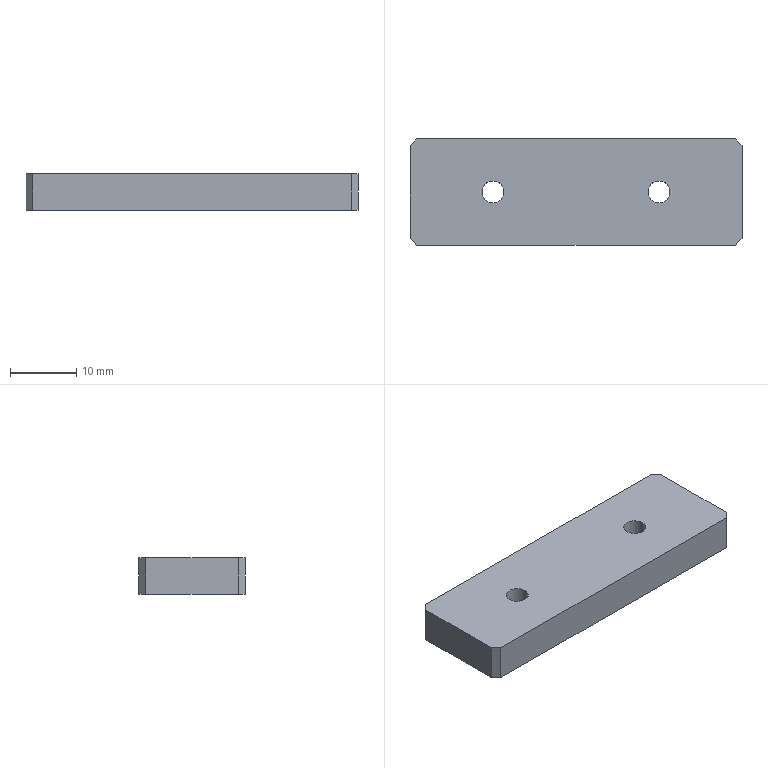Part | SolidWorks | features Chamfer 1, Extrusion 1, HoleWzd 1 | 1 solid | 14 faces | box 50 x 16 x 5.5 mm | volume 4295 mm3 | plane 10 | cylinder 4 | commonest cylinder face diameters 3.3 x4
STEP:
#1=CARTESIAN_POINT('',(-10.85,0.,2.75));
#2=VERTEX_POINT('',#1);
#3=CARTESIAN_POINT('',(-14.15,0.,2.75));
#4=VERTEX_POINT('',#3);
#5=CARTESIAN_POINT('',(-12.5,0.,2.75));
#6=DIRECTION('',(0.,0.,-1.));
#7=DIRECTION('',(-1.,0.,0.));
#8=AXIS2_PLACEMENT_3D('',#5,#6,#7);
#9=CIRCLE('',#8,1.65);
#10=EDGE_CURVE('',#2,#4,#9,.T.);
#11=ORIENTED_EDGE('',*,*,#10,.F.);
#12=CARTESIAN_POINT('',(-10.85,0.,-2.75));
#13=VERTEX_POINT('',#12);
#14=CARTESIAN_POINT('',(-10.85,0.,-2.75));
#15=DIRECTION('',(0.,0.,-1.));
#16=VECTOR('',#15,1000.);
#17=LINE('',#14,#16);
#18=EDGE_CURVE('',#2,#13,#17,.T.);
#19=ORIENTED_EDGE('',*,*,#18,.T.);
#20=CARTESIAN_POINT('',(-14.15,0.,-2.75));
#21=VERTEX_POINT('',#20);
#22=CARTESIAN_POINT('',(-12.5,0.,-2.75));
#23=DIRECTION('',(0.,0.,-1.));
#24=DIRECTION('',(-1.,0.,0.));
#25=AXIS2_PLACEMENT_3D('',#22,#23,#24);
#26=CIRCLE('',#25,1.65);
#27=EDGE_CURVE('',#13,#21,#26,.T.);
#28=ORIENTED_EDGE('',*,*,#27,.T.);
#29=CARTESIAN_POINT('',(-14.15,0.,-2.75));
#30=DIRECTION('',(0.,0.,-1.));
#31=VECTOR('',#30,1000.);
#32=LINE('',#29,#31);
#33=EDGE_CURVE('',#4,#21,#32,.T.);
#34=ORIENTED_EDGE('',*,*,#33,.F.);
#35=EDGE_LOOP('',(#11,#19,#28,#34));
#36=FACE_OUTER_BOUND('',#35,.T.);
#37=CARTESIAN_POINT('',(-12.5,0.,-2.75));
#38=DIRECTION('',(0.,0.,-1.));
#39=DIRECTION('',(-1.,0.,0.));
#40=AXIS2_PLACEMENT_3D('',#37,#38,#39);
#41=CYLINDRICAL_SURFACE('',#40,1.65);
#42=ADVANCED_FACE('',(#36),#41,.F.);
#43=CARTESIAN_POINT('',(14.15,0.,2.75));
#44=VERTEX_POINT('',#43);
#45=CARTESIAN_POINT('',(10.85,0.,2.75));
#46=VERTEX_POINT('',#45);
#47=CARTESIAN_POINT('',(12.5,0.,2.75));
#48=DIRECTION('',(0.,0.,-1.));
#49=DIRECTION('',(-1.,0.,0.));
#50=AXIS2_PLACEMENT_3D('',#47,#48,#49);
#51=CIRCLE('',#50,1.65);
#52=EDGE_CURVE('',#44,#46,#51,.T.);
#53=ORIENTED_EDGE('',*,*,#52,.F.);
#54=CARTESIAN_POINT('',(14.15,0.,-2.75));
#55=VERTEX_POINT('',#54);
#56=CARTESIAN_POINT('',(14.15,0.,-2.75));
#57=DIRECTION('',(0.,0.,-1.));
#58=VECTOR('',#57,1000.);
#59=LINE('',#56,#58);
#60=EDGE_CURVE('',#44,#55,#59,.T.);
#61=ORIENTED_EDGE('',*,*,#60,.T.);
#62=CARTESIAN_POINT('',(10.85,0.,-2.75));
#63=VERTEX_POINT('',#62);
#64=CARTESIAN_POINT('',(12.5,0.,-2.75));
#65=DIRECTION('',(0.,0.,-1.));
#66=DIRECTION('',(-1.,0.,0.));
#67=AXIS2_PLACEMENT_3D('',#64,#65,#66);
#68=CIRCLE('',#67,1.65);
#69=EDGE_CURVE('',#55,#63,#68,.T.);
#70=ORIENTED_EDGE('',*,*,#69,.T.);
#71=CARTESIAN_POINT('',(10.85,0.,-2.75));
#72=DIRECTION('',(0.,0.,-1.));
#73=VECTOR('',#72,1000.);
#74=LINE('',#71,#73);
#75=EDGE_CURVE('',#46,#63,#74,.T.);
#76=ORIENTED_EDGE('',*,*,#75,.F.);
#77=EDGE_LOOP('',(#53,#61,#70,#76));
#78=FACE_OUTER_BOUND('',#77,.T.);
#79=CARTESIAN_POINT('',(12.5,0.,-2.75));
#80=DIRECTION('',(0.,0.,-1.));
#81=DIRECTION('',(-1.,0.,0.));
#82=AXIS2_PLACEMENT_3D('',#79,#80,#81);
#83=CYLINDRICAL_SURFACE('',#82,1.65);
#84=ADVANCED_FACE('',(#78),#83,.F.);
#85=CARTESIAN_POINT('',(25.,-7.,2.75));
#86=VERTEX_POINT('',#85);
#87=CARTESIAN_POINT('',(25.,7.,2.75));
#88=VERTEX_POINT('',#87);
#89=CARTESIAN_POINT('',(25.,8.,2.75));
#90=DIRECTION('',(0.,1.,0.));
#91=VECTOR('',#90,1000.);
#92=LINE('',#89,#91);
#93=EDGE_CURVE('',#86,#88,#92,.T.);
#94=ORIENTED_EDGE('',*,*,#93,.F.);
#95=CARTESIAN_POINT('',(25.,-7.,-2.75));
#96=VERTEX_POINT('',#95);
#97=CARTESIAN_POINT('',(25.,-7.,2.75));
#98=DIRECTION('',(0.,0.,-1.));
#99=VECTOR('',#98,1000.);
#100=LINE('',#97,#99);
#101=EDGE_CURVE('',#86,#96,#100,.T.);
#102=ORIENTED_EDGE('',*,*,#101,.T.);
#103=CARTESIAN_POINT('',(25.,7.,-2.75));
#104=VERTEX_POINT('',#103);
#105=CARTESIAN_POINT('',(25.,8.,-2.75));
#106=DIRECTION('',(0.,1.,0.));
#107=VECTOR('',#106,1000.);
#108=LINE('',#105,#107);
#109=EDGE_CURVE('',#96,#104,#108,.T.);
#110=ORIENTED_EDGE('',*,*,#109,.T.);
#111=CARTESIAN_POINT('',(25.,7.,2.75));
#112=DIRECTION('',(0.,0.,1.));
#113=VECTOR('',#112,1000.);
#114=LINE('',#111,#113);
#115=EDGE_CURVE('',#104,#88,#114,.T.);
#116=ORIENTED_EDGE('',*,*,#115,.T.);
#117=EDGE_LOOP('',(#94,#102,#110,#116));
#118=FACE_OUTER_BOUND('',#117,.T.);
#119=CARTESIAN_POINT('',(25.,8.,2.75));
#120=DIRECTION('',(-1.,0.,0.));
#121=DIRECTION('',(0.,-1.,0.));
#122=AXIS2_PLACEMENT_3D('',#119,#120,#121);
#123=PLANE('',#122);
#124=ADVANCED_FACE('',(#118),#123,.F.);
#125=CARTESIAN_POINT('',(24.,8.,-2.75));
#126=VERTEX_POINT('',#125);
#127=CARTESIAN_POINT('',(-24.,8.,-2.75));
#128=VERTEX_POINT('',#127);
#129=CARTESIAN_POINT('',(-25.,8.,-2.75));
#130=DIRECTION('',(-1.,0.,0.));
#131=VECTOR('',#130,1000.);
#132=LINE('',#129,#131);
#133=EDGE_CURVE('',#126,#128,#132,.T.);
#134=ORIENTED_EDGE('',*,*,#133,.T.);
#135=CARTESIAN_POINT('',(-24.,8.,2.75));
#136=VERTEX_POINT('',#135);
#137=CARTESIAN_POINT('',(-24.,8.,2.75));
#138=DIRECTION('',(0.,0.,1.));
#139=VECTOR('',#138,1000.);
#140=LINE('',#137,#139);
#141=EDGE_CURVE('',#128,#136,#140,.T.);
#142=ORIENTED_EDGE('',*,*,#141,.T.);
#143=CARTESIAN_POINT('',(24.,8.,2.75));
#144=VERTEX_POINT('',#143);
#145=CARTESIAN_POINT('',(-25.,8.,2.75));
#146=DIRECTION('',(-1.,0.,0.));
#147=VECTOR('',#146,1000.);
#148=LINE('',#145,#147);
#149=EDGE_CURVE('',#144,#136,#148,.T.);
#150=ORIENTED_EDGE('',*,*,#149,.F.);
#151=CARTESIAN_POINT('',(24.,8.,2.75));
#152=DIRECTION('',(0.,0.,-1.));
#153=VECTOR('',#152,1000.);
#154=LINE('',#151,#153);
#155=EDGE_CURVE('',#144,#126,#154,.T.);
#156=ORIENTED_EDGE('',*,*,#155,.T.);
#157=EDGE_LOOP('',(#134,#142,#150,#156));
#158=FACE_OUTER_BOUND('',#157,.T.);
#159=CARTESIAN_POINT('',(-25.,8.,2.75));
#160=DIRECTION('',(0.,-1.,0.));
#161=DIRECTION('',(0.,0.,-1.));
#162=AXIS2_PLACEMENT_3D('',#159,#160,#161);
#163=PLANE('',#162);
#164=ADVANCED_FACE('',(#158),#163,.F.);
#165=CARTESIAN_POINT('',(-25.,7.,-2.75));
#166=VERTEX_POINT('',#165);
#167=CARTESIAN_POINT('',(-25.,-7.,-2.75));
#168=VERTEX_POINT('',#167);
#169=CARTESIAN_POINT('',(-25.,8.,-2.75));
#170=DIRECTION('',(0.,-1.,0.));
#171=VECTOR('',#170,1000.);
#172=LINE('',#169,#171);
#173=EDGE_CURVE('',#166,#168,#172,.T.);
#174=ORIENTED_EDGE('',*,*,#173,.T.);
#175=CARTESIAN_POINT('',(-25.,-7.,2.75));
#176=VERTEX_POINT('',#175);
#177=CARTESIAN_POINT('',(-25.,-7.,2.75));
#178=DIRECTION('',(0.,0.,1.));
#179=VECTOR('',#178,1000.);
#180=LINE('',#177,#179);
#181=EDGE_CURVE('',#168,#176,#180,.T.);
#182=ORIENTED_EDGE('',*,*,#181,.T.);
#183=CARTESIAN_POINT('',(-25.,7.,2.75));
#184=VERTEX_POINT('',#183);
#185=CARTESIAN_POINT('',(-25.,8.,2.75));
#186=DIRECTION('',(0.,-1.,0.));
#187=VECTOR('',#186,1000.);
#188=LINE('',#185,#187);
#189=EDGE_CURVE('',#184,#176,#188,.T.);
#190=ORIENTED_EDGE('',*,*,#189,.F.);
#191=CARTESIAN_POINT('',(-25.,7.,2.75));
#192=DIRECTION('',(0.,0.,-1.));
#193=VECTOR('',#192,1000.);
#194=LINE('',#191,#193);
#195=EDGE_CURVE('',#184,#166,#194,.T.);
#196=ORIENTED_EDGE('',*,*,#195,.T.);
#197=EDGE_LOOP('',(#174,#182,#190,#196));
#198=FACE_OUTER_BOUND('',#197,.T.);
#199=CARTESIAN_POINT('',(-25.,8.,2.75));
#200=DIRECTION('',(1.,0.,0.));
#201=DIRECTION('',(0.,0.,-1.));
#202=AXIS2_PLACEMENT_3D('',#199,#200,#201);
#203=PLANE('',#202);
#204=ADVANCED_FACE('',(#198),#203,.F.);
#205=CARTESIAN_POINT('',(-24.,-8.,2.75));
#206=VERTEX_POINT('',#205);
#207=CARTESIAN_POINT('',(24.,-8.,2.75));
#208=VERTEX_POINT('',#207);
#209=CARTESIAN_POINT('',(-25.,-8.,2.75));
#210=DIRECTION('',(1.,0.,0.));
#211=VECTOR('',#210,1000.);
#212=LINE('',#209,#211);
#213=EDGE_CURVE('',#206,#208,#212,.T.);
#214=ORIENTED_EDGE('',*,*,#213,.F.);
#215=CARTESIAN_POINT('',(-24.,-8.,-2.75));
#216=VERTEX_POINT('',#215);
#217=CARTESIAN_POINT('',(-24.,-8.,2.75));
#218=DIRECTION('',(0.,0.,-1.));
#219=VECTOR('',#218,1000.);
#220=LINE('',#217,#219);
#221=EDGE_CURVE('',#206,#216,#220,.T.);
#222=ORIENTED_EDGE('',*,*,#221,.T.);
#223=CARTESIAN_POINT('',(24.,-8.,-2.75));
#224=VERTEX_POINT('',#223);
#225=CARTESIAN_POINT('',(-25.,-8.,-2.75));
#226=DIRECTION('',(1.,0.,0.));
#227=VECTOR('',#226,1000.);
#228=LINE('',#225,#227);
#229=EDGE_CURVE('',#216,#224,#228,.T.);
#230=ORIENTED_EDGE('',*,*,#229,.T.);
#231=CARTESIAN_POINT('',(24.,-8.,2.75));
#232=DIRECTION('',(0.,0.,1.));
#233=VECTOR('',#232,1000.);
#234=LINE('',#231,#233);
#235=EDGE_CURVE('',#224,#208,#234,.T.);
#236=ORIENTED_EDGE('',*,*,#235,.T.);
#237=EDGE_LOOP('',(#214,#222,#230,#236));
#238=FACE_OUTER_BOUND('',#237,.T.);
#239=CARTESIAN_POINT('',(-25.,-8.,2.75));
#240=DIRECTION('',(0.,1.,0.));
#241=DIRECTION('',(0.,0.,1.));
#242=AXIS2_PLACEMENT_3D('',#239,#240,#241);
#243=PLANE('',#242);
#244=ADVANCED_FACE('',(#238),#243,.F.);
#245=CARTESIAN_POINT('',(-12.5,0.,2.75));
#246=DIRECTION('',(0.,0.,-1.));
#247=DIRECTION('',(-1.,0.,0.));
#248=AXIS2_PLACEMENT_3D('',#245,#246,#247);
#249=CIRCLE('',#248,1.65);
#250=EDGE_CURVE('',#4,#2,#249,.T.);
#251=ORIENTED_EDGE('',*,*,#250,.T.);
#252=ORIENTED_EDGE('',*,*,#10,.T.);
#253=EDGE_LOOP('',(#251,#252));
#254=FACE_BOUND('',#253,.T.);
#255=CARTESIAN_POINT('',(12.5,0.,2.75));
#256=DIRECTION('',(0.,0.,-1.));
#257=DIRECTION('',(-1.,0.,0.));
#258=AXIS2_PLACEMENT_3D('',#255,#256,#257);
#259=CIRCLE('',#258,1.65);
#260=EDGE_CURVE('',#46,#44,#259,.T.);
#261=ORIENTED_EDGE('',*,*,#260,.T.);
#262=ORIENTED_EDGE('',*,*,#52,.T.);
#263=EDGE_LOOP('',(#261,#262));
#264=FACE_BOUND('',#263,.T.);
#265=ORIENTED_EDGE('',*,*,#189,.T.);
#266=CARTESIAN_POINT('',(-16.,-16.,2.75));
#267=DIRECTION('',(0.7071,-0.7071,0.));
#268=VECTOR('',#267,1000.);
#269=LINE('',#266,#268);
#270=EDGE_CURVE('',#176,#206,#269,.T.);
#271=ORIENTED_EDGE('',*,*,#270,.T.);
#272=ORIENTED_EDGE('',*,*,#213,.T.);
#273=CARTESIAN_POINT('',(16.,-16.,2.75));
#274=DIRECTION('',(0.7071,0.7071,0.));
#275=VECTOR('',#274,1000.);
#276=LINE('',#273,#275);
#277=EDGE_CURVE('',#208,#86,#276,.T.);
#278=ORIENTED_EDGE('',*,*,#277,.T.);
#279=ORIENTED_EDGE('',*,*,#93,.T.);
#280=CARTESIAN_POINT('',(16.,16.,2.75));
#281=DIRECTION('',(-0.7071,0.7071,0.));
#282=VECTOR('',#281,1000.);
#283=LINE('',#280,#282);
#284=EDGE_CURVE('',#88,#144,#283,.T.);
#285=ORIENTED_EDGE('',*,*,#284,.T.);
#286=ORIENTED_EDGE('',*,*,#149,.T.);
#287=CARTESIAN_POINT('',(-16.,16.,2.75));
#288=DIRECTION('',(-0.7071,-0.7071,0.));
#289=VECTOR('',#288,1000.);
#290=LINE('',#287,#289);
#291=EDGE_CURVE('',#136,#184,#290,.T.);
#292=ORIENTED_EDGE('',*,*,#291,.T.);
#293=EDGE_LOOP('',(#265,#271,#272,#278,#279,#285,#286,#292));
#294=FACE_OUTER_BOUND('',#293,.T.);
#295=CARTESIAN_POINT('',(0.,0.,2.75));
#296=DIRECTION('',(0.,0.,1.));
#297=DIRECTION('',(1.,0.,0.));
#298=AXIS2_PLACEMENT_3D('',#295,#296,#297);
#299=PLANE('',#298);
#300=ADVANCED_FACE('',(#254,#264,#294),#299,.T.);
#301=CARTESIAN_POINT('',(-12.5,0.,-2.75));
#302=DIRECTION('',(0.,0.,-1.));
#303=DIRECTION('',(-1.,0.,0.));
#304=AXIS2_PLACEMENT_3D('',#301,#302,#303);
#305=CIRCLE('',#304,1.65);
#306=EDGE_CURVE('',#21,#13,#305,.T.);
#307=ORIENTED_EDGE('',*,*,#306,.F.);
#308=ORIENTED_EDGE('',*,*,#27,.F.);
#309=EDGE_LOOP('',(#307,#308));
#310=FACE_BOUND('',#309,.T.);
#311=CARTESIAN_POINT('',(12.5,0.,-2.75));
#312=DIRECTION('',(0.,0.,-1.));
#313=DIRECTION('',(-1.,0.,0.));
#314=AXIS2_PLACEMENT_3D('',#311,#312,#313);
#315=CIRCLE('',#314,1.65);
#316=EDGE_CURVE('',#63,#55,#315,.T.);
#317=ORIENTED_EDGE('',*,*,#316,.F.);
#318=ORIENTED_EDGE('',*,*,#69,.F.);
#319=EDGE_LOOP('',(#317,#318));
#320=FACE_BOUND('',#319,.T.);
#321=ORIENTED_EDGE('',*,*,#229,.F.);
#322=CARTESIAN_POINT('',(-24.,-8.,-2.75));
#323=DIRECTION('',(-0.7071,0.7071,0.));
#324=VECTOR('',#323,1000.);
#325=LINE('',#322,#324);
#326=EDGE_CURVE('',#216,#168,#325,.T.);
#327=ORIENTED_EDGE('',*,*,#326,.T.);
#328=ORIENTED_EDGE('',*,*,#173,.F.);
#329=CARTESIAN_POINT('',(-25.,7.,-2.75));
#330=DIRECTION('',(0.7071,0.7071,0.));
#331=VECTOR('',#330,1000.);
#332=LINE('',#329,#331);
#333=EDGE_CURVE('',#166,#128,#332,.T.);
#334=ORIENTED_EDGE('',*,*,#333,.T.);
#335=ORIENTED_EDGE('',*,*,#133,.F.);
#336=CARTESIAN_POINT('',(24.,8.,-2.75));
#337=DIRECTION('',(0.7071,-0.7071,0.));
#338=VECTOR('',#337,1000.);
#339=LINE('',#336,#338);
#340=EDGE_CURVE('',#126,#104,#339,.T.);
#341=ORIENTED_EDGE('',*,*,#340,.T.);
#342=ORIENTED_EDGE('',*,*,#109,.F.);
#343=CARTESIAN_POINT('',(25.,-7.,-2.75));
#344=DIRECTION('',(-0.7071,-0.7071,0.));
#345=VECTOR('',#344,1000.);
#346=LINE('',#343,#345);
#347=EDGE_CURVE('',#96,#224,#346,.T.);
#348=ORIENTED_EDGE('',*,*,#347,.T.);
#349=EDGE_LOOP('',(#321,#327,#328,#334,#335,#341,#342,#348));
#350=FACE_OUTER_BOUND('',#349,.T.);
#351=CARTESIAN_POINT('',(0.,0.,-2.75));
#352=DIRECTION('',(0.,0.,1.));
#353=DIRECTION('',(1.,0.,0.));
#354=AXIS2_PLACEMENT_3D('',#351,#352,#353);
#355=PLANE('',#354);
#356=ADVANCED_FACE('',(#310,#320,#350),#355,.F.);
#357=ORIENTED_EDGE('',*,*,#60,.F.);
#358=ORIENTED_EDGE('',*,*,#260,.F.);
#359=ORIENTED_EDGE('',*,*,#75,.T.);
#360=ORIENTED_EDGE('',*,*,#316,.T.);
#361=EDGE_LOOP('',(#357,#358,#359,#360));
#362=FACE_OUTER_BOUND('',#361,.T.);
#363=CARTESIAN_POINT('',(12.5,0.,-2.75));
#364=DIRECTION('',(0.,0.,-1.));
#365=DIRECTION('',(-1.,0.,0.));
#366=AXIS2_PLACEMENT_3D('',#363,#364,#365);
#367=CYLINDRICAL_SURFACE('',#366,1.65);
#368=ADVANCED_FACE('',(#362),#367,.F.);
#369=ORIENTED_EDGE('',*,*,#18,.F.);
#370=ORIENTED_EDGE('',*,*,#250,.F.);
#371=ORIENTED_EDGE('',*,*,#33,.T.);
#372=ORIENTED_EDGE('',*,*,#306,.T.);
#373=EDGE_LOOP('',(#369,#370,#371,#372));
#374=FACE_OUTER_BOUND('',#373,.T.);
#375=CARTESIAN_POINT('',(-12.5,0.,-2.75));
#376=DIRECTION('',(0.,0.,-1.));
#377=DIRECTION('',(-1.,0.,0.));
#378=AXIS2_PLACEMENT_3D('',#375,#376,#377);
#379=CYLINDRICAL_SURFACE('',#378,1.65);
#380=ADVANCED_FACE('',(#374),#379,.F.);
#381=ORIENTED_EDGE('',*,*,#270,.F.);
#382=ORIENTED_EDGE('',*,*,#181,.F.);
#383=ORIENTED_EDGE('',*,*,#326,.F.);
#384=ORIENTED_EDGE('',*,*,#221,.F.);
#385=EDGE_LOOP('',(#381,#382,#383,#384));
#386=FACE_OUTER_BOUND('',#385,.T.);
#387=CARTESIAN_POINT('',(-24.,-8.,2.75));
#388=DIRECTION('',(0.7071,0.7071,0.));
#389=DIRECTION('',(0.,0.,-1.));
#390=AXIS2_PLACEMENT_3D('',#387,#388,#389);
#391=PLANE('',#390);
#392=ADVANCED_FACE('',(#386),#391,.F.);
#393=ORIENTED_EDGE('',*,*,#291,.F.);
#394=ORIENTED_EDGE('',*,*,#141,.F.);
#395=ORIENTED_EDGE('',*,*,#333,.F.);
#396=ORIENTED_EDGE('',*,*,#195,.F.);
#397=EDGE_LOOP('',(#393,#394,#395,#396));
#398=FACE_OUTER_BOUND('',#397,.T.);
#399=CARTESIAN_POINT('',(-25.,7.,2.75));
#400=DIRECTION('',(0.7071,-0.7071,0.));
#401=DIRECTION('',(0.,0.,-1.));
#402=AXIS2_PLACEMENT_3D('',#399,#400,#401);
#403=PLANE('',#402);
#404=ADVANCED_FACE('',(#398),#403,.F.);
#405=ORIENTED_EDGE('',*,*,#277,.F.);
#406=ORIENTED_EDGE('',*,*,#235,.F.);
#407=ORIENTED_EDGE('',*,*,#347,.F.);
#408=ORIENTED_EDGE('',*,*,#101,.F.);
#409=EDGE_LOOP('',(#405,#406,#407,#408));
#410=FACE_OUTER_BOUND('',#409,.T.);
#411=CARTESIAN_POINT('',(25.,-7.,2.75));
#412=DIRECTION('',(-0.7071,0.7071,0.));
#413=DIRECTION('',(0.,0.,-1.));
#414=AXIS2_PLACEMENT_3D('',#411,#412,#413);
#415=PLANE('',#414);
#416=ADVANCED_FACE('',(#410),#415,.F.);
#417=ORIENTED_EDGE('',*,*,#284,.F.);
#418=ORIENTED_EDGE('',*,*,#115,.F.);
#419=ORIENTED_EDGE('',*,*,#340,.F.);
#420=ORIENTED_EDGE('',*,*,#155,.F.);
#421=EDGE_LOOP('',(#417,#418,#419,#420));
#422=FACE_OUTER_BOUND('',#421,.T.);
#423=CARTESIAN_POINT('',(24.,8.,2.75));
#424=DIRECTION('',(-0.7071,-0.7071,0.));
#425=DIRECTION('',(0.,0.,-1.));
#426=AXIS2_PLACEMENT_3D('',#423,#424,#425);
#427=PLANE('',#426);
#428=ADVANCED_FACE('',(#422),#427,.F.);
#429=CLOSED_SHELL('',(#42,#84,#124,#164,#204,#244,#300,#356,#368,#380,#392,#404,#416,#428));
#430=MANIFOLD_SOLID_BREP('',#429);
#431=CARTESIAN_POINT('',(0.,0.,0.));
#432=DIRECTION('',(0.,0.,1.));
#433=DIRECTION('',(1.,0.,0.));
#434=AXIS2_PLACEMENT_3D('',#431,#432,#433);
#435=(LENGTH_UNIT()NAMED_UNIT(*)SI_UNIT(.MILLI.,.METRE.));
#436=UNCERTAINTY_MEASURE_WITH_UNIT(LENGTH_MEASURE(0.00001),#435,'','');
#437=(NAMED_UNIT(*)PLANE_ANGLE_UNIT()SI_UNIT($,.RADIAN.));
#438=(NAMED_UNIT(*)SI_UNIT($,.STERADIAN.)SOLID_ANGLE_UNIT());
#439=(GEOMETRIC_REPRESENTATION_CONTEXT(3)GLOBAL_UNCERTAINTY_ASSIGNED_CONTEXT((#436))GLOBAL_UNIT_ASSIGNED_CONTEXT((#435,#437,#438))REPRESENTATION_CONTEXT('',''));
#440=ADVANCED_BREP_SHAPE_REPRESENTATION('',(#430,#434),#439);